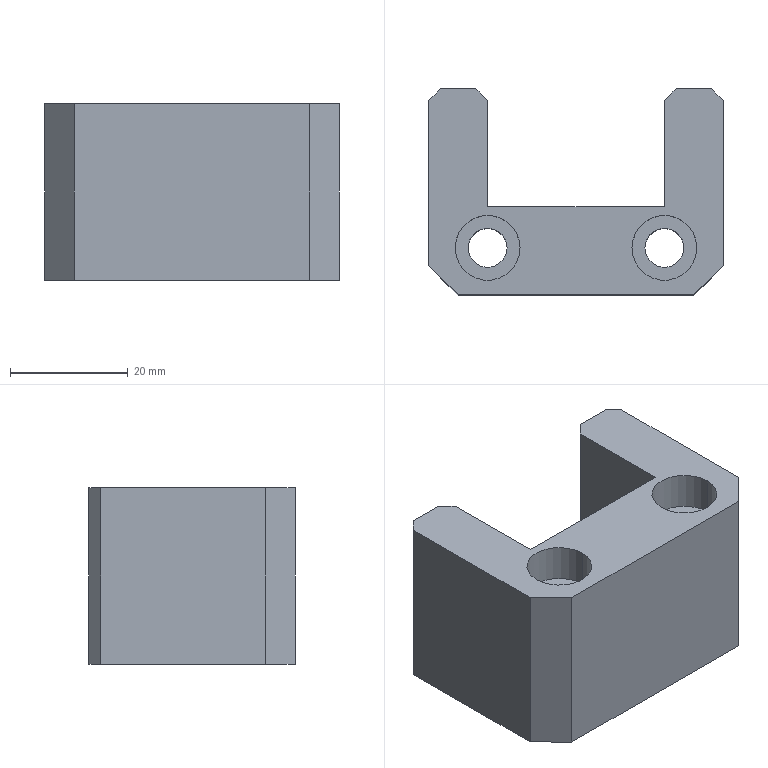Part | SolidWorks | features Chamfer 2, Extrusion 1, HoleWzd 1 | 1 solid | 26 faces | box 50 x 35 x 30 mm | volume 30679 mm3 | plane 18 | cylinder 8 | commonest cylinder face diameters 6.6 x4 11 x4
STEP:
#1=CARTESIAN_POINT('',(-20.5,-7.,23.6));
#2=VERTEX_POINT('',#1);
#3=CARTESIAN_POINT('',(-9.5,-7.,23.6));
#4=VERTEX_POINT('',#3);
#5=CARTESIAN_POINT('',(-15.,-7.,23.6));
#6=DIRECTION('',(0.,0.,1.));
#7=DIRECTION('',(1.,0.,0.));
#8=AXIS2_PLACEMENT_3D('',#5,#6,#7);
#9=CIRCLE('',#8,5.5);
#10=EDGE_CURVE('',#2,#4,#9,.T.);
#11=ORIENTED_EDGE('',*,*,#10,.F.);
#12=CARTESIAN_POINT('',(-20.5,-7.,30.));
#13=VERTEX_POINT('',#12);
#14=CARTESIAN_POINT('',(-20.5,-7.,30.));
#15=DIRECTION('',(0.,0.,1.));
#16=VECTOR('',#15,1000.);
#17=LINE('',#14,#16);
#18=EDGE_CURVE('',#2,#13,#17,.T.);
#19=ORIENTED_EDGE('',*,*,#18,.T.);
#20=CARTESIAN_POINT('',(-9.5,-7.,30.));
#21=VERTEX_POINT('',#20);
#22=CARTESIAN_POINT('',(-15.,-7.,30.));
#23=DIRECTION('',(0.,0.,1.));
#24=DIRECTION('',(1.,0.,0.));
#25=AXIS2_PLACEMENT_3D('',#22,#23,#24);
#26=CIRCLE('',#25,5.5);
#27=EDGE_CURVE('',#13,#21,#26,.T.);
#28=ORIENTED_EDGE('',*,*,#27,.T.);
#29=CARTESIAN_POINT('',(-9.5,-7.,30.));
#30=DIRECTION('',(0.,0.,1.));
#31=VECTOR('',#30,1000.);
#32=LINE('',#29,#31);
#33=EDGE_CURVE('',#4,#21,#32,.T.);
#34=ORIENTED_EDGE('',*,*,#33,.F.);
#35=EDGE_LOOP('',(#11,#19,#28,#34));
#36=FACE_OUTER_BOUND('',#35,.T.);
#37=CARTESIAN_POINT('',(-15.,-7.,30.));
#38=DIRECTION('',(0.,0.,1.));
#39=DIRECTION('',(1.,0.,0.));
#40=AXIS2_PLACEMENT_3D('',#37,#38,#39);
#41=CYLINDRICAL_SURFACE('',#40,5.5);
#42=ADVANCED_FACE('',(#36),#41,.F.);
#43=CARTESIAN_POINT('',(-18.3,-7.,0.));
#44=VERTEX_POINT('',#43);
#45=CARTESIAN_POINT('',(-11.7,-7.,0.));
#46=VERTEX_POINT('',#45);
#47=CARTESIAN_POINT('',(-15.,-7.,0.));
#48=DIRECTION('',(0.,0.,1.));
#49=DIRECTION('',(1.,0.,0.));
#50=AXIS2_PLACEMENT_3D('',#47,#48,#49);
#51=CIRCLE('',#50,3.3);
#52=EDGE_CURVE('',#44,#46,#51,.T.);
#53=ORIENTED_EDGE('',*,*,#52,.F.);
#54=CARTESIAN_POINT('',(-18.3,-7.,23.6));
#55=VERTEX_POINT('',#54);
#56=CARTESIAN_POINT('',(-18.3,-7.,30.));
#57=DIRECTION('',(0.,0.,1.));
#58=VECTOR('',#57,1000.);
#59=LINE('',#56,#58);
#60=EDGE_CURVE('',#44,#55,#59,.T.);
#61=ORIENTED_EDGE('',*,*,#60,.T.);
#62=CARTESIAN_POINT('',(-11.7,-7.,23.6));
#63=VERTEX_POINT('',#62);
#64=CARTESIAN_POINT('',(-15.,-7.,23.6));
#65=DIRECTION('',(0.,0.,1.));
#66=DIRECTION('',(1.,0.,0.));
#67=AXIS2_PLACEMENT_3D('',#64,#65,#66);
#68=CIRCLE('',#67,3.3);
#69=EDGE_CURVE('',#55,#63,#68,.T.);
#70=ORIENTED_EDGE('',*,*,#69,.T.);
#71=CARTESIAN_POINT('',(-11.7,-7.,30.));
#72=DIRECTION('',(0.,0.,1.));
#73=VECTOR('',#72,1000.);
#74=LINE('',#71,#73);
#75=EDGE_CURVE('',#46,#63,#74,.T.);
#76=ORIENTED_EDGE('',*,*,#75,.F.);
#77=EDGE_LOOP('',(#53,#61,#70,#76));
#78=FACE_OUTER_BOUND('',#77,.T.);
#79=CARTESIAN_POINT('',(-15.,-7.,30.));
#80=DIRECTION('',(0.,0.,1.));
#81=DIRECTION('',(1.,0.,0.));
#82=AXIS2_PLACEMENT_3D('',#79,#80,#81);
#83=CYLINDRICAL_SURFACE('',#82,3.3);
#84=ADVANCED_FACE('',(#78),#83,.F.);
#85=CARTESIAN_POINT('',(9.5,-7.,23.6));
#86=VERTEX_POINT('',#85);
#87=CARTESIAN_POINT('',(20.5,-7.,23.6));
#88=VERTEX_POINT('',#87);
#89=CARTESIAN_POINT('',(15.,-7.,23.6));
#90=DIRECTION('',(0.,0.,1.));
#91=DIRECTION('',(1.,0.,0.));
#92=AXIS2_PLACEMENT_3D('',#89,#90,#91);
#93=CIRCLE('',#92,5.5);
#94=EDGE_CURVE('',#86,#88,#93,.T.);
#95=ORIENTED_EDGE('',*,*,#94,.F.);
#96=CARTESIAN_POINT('',(9.5,-7.,30.));
#97=VERTEX_POINT('',#96);
#98=CARTESIAN_POINT('',(9.5,-7.,30.));
#99=DIRECTION('',(0.,0.,1.));
#100=VECTOR('',#99,1000.);
#101=LINE('',#98,#100);
#102=EDGE_CURVE('',#86,#97,#101,.T.);
#103=ORIENTED_EDGE('',*,*,#102,.T.);
#104=CARTESIAN_POINT('',(20.5,-7.,30.));
#105=VERTEX_POINT('',#104);
#106=CARTESIAN_POINT('',(15.,-7.,30.));
#107=DIRECTION('',(0.,0.,1.));
#108=DIRECTION('',(1.,0.,0.));
#109=AXIS2_PLACEMENT_3D('',#106,#107,#108);
#110=CIRCLE('',#109,5.5);
#111=EDGE_CURVE('',#97,#105,#110,.T.);
#112=ORIENTED_EDGE('',*,*,#111,.T.);
#113=CARTESIAN_POINT('',(20.5,-7.,30.));
#114=DIRECTION('',(0.,0.,1.));
#115=VECTOR('',#114,1000.);
#116=LINE('',#113,#115);
#117=EDGE_CURVE('',#88,#105,#116,.T.);
#118=ORIENTED_EDGE('',*,*,#117,.F.);
#119=EDGE_LOOP('',(#95,#103,#112,#118));
#120=FACE_OUTER_BOUND('',#119,.T.);
#121=CARTESIAN_POINT('',(15.,-7.,30.));
#122=DIRECTION('',(0.,0.,1.));
#123=DIRECTION('',(1.,0.,0.));
#124=AXIS2_PLACEMENT_3D('',#121,#122,#123);
#125=CYLINDRICAL_SURFACE('',#124,5.5);
#126=ADVANCED_FACE('',(#120),#125,.F.);
#127=CARTESIAN_POINT('',(11.7,-7.,0.));
#128=VERTEX_POINT('',#127);
#129=CARTESIAN_POINT('',(18.3,-7.,0.));
#130=VERTEX_POINT('',#129);
#131=CARTESIAN_POINT('',(15.,-7.,0.));
#132=DIRECTION('',(0.,0.,1.));
#133=DIRECTION('',(1.,0.,0.));
#134=AXIS2_PLACEMENT_3D('',#131,#132,#133);
#135=CIRCLE('',#134,3.3);
#136=EDGE_CURVE('',#128,#130,#135,.T.);
#137=ORIENTED_EDGE('',*,*,#136,.F.);
#138=CARTESIAN_POINT('',(11.7,-7.,23.6));
#139=VERTEX_POINT('',#138);
#140=CARTESIAN_POINT('',(11.7,-7.,30.));
#141=DIRECTION('',(0.,0.,1.));
#142=VECTOR('',#141,1000.);
#143=LINE('',#140,#142);
#144=EDGE_CURVE('',#128,#139,#143,.T.);
#145=ORIENTED_EDGE('',*,*,#144,.T.);
#146=CARTESIAN_POINT('',(18.3,-7.,23.6));
#147=VERTEX_POINT('',#146);
#148=CARTESIAN_POINT('',(15.,-7.,23.6));
#149=DIRECTION('',(0.,0.,1.));
#150=DIRECTION('',(1.,0.,0.));
#151=AXIS2_PLACEMENT_3D('',#148,#149,#150);
#152=CIRCLE('',#151,3.3);
#153=EDGE_CURVE('',#139,#147,#152,.T.);
#154=ORIENTED_EDGE('',*,*,#153,.T.);
#155=CARTESIAN_POINT('',(18.3,-7.,30.));
#156=DIRECTION('',(0.,0.,1.));
#157=VECTOR('',#156,1000.);
#158=LINE('',#155,#157);
#159=EDGE_CURVE('',#130,#147,#158,.T.);
#160=ORIENTED_EDGE('',*,*,#159,.F.);
#161=EDGE_LOOP('',(#137,#145,#154,#160));
#162=FACE_OUTER_BOUND('',#161,.T.);
#163=CARTESIAN_POINT('',(15.,-7.,30.));
#164=DIRECTION('',(0.,0.,1.));
#165=DIRECTION('',(1.,0.,0.));
#166=AXIS2_PLACEMENT_3D('',#163,#164,#165);
#167=CYLINDRICAL_SURFACE('',#166,3.3);
#168=ADVANCED_FACE('',(#162),#167,.F.);
#169=CARTESIAN_POINT('',(-25.,18.,0.));
#170=VERTEX_POINT('',#169);
#171=CARTESIAN_POINT('',(-25.,-10.,0.));
#172=VERTEX_POINT('',#171);
#173=CARTESIAN_POINT('',(-25.,-15.,0.));
#174=DIRECTION('',(0.,-1.,0.));
#175=VECTOR('',#174,1000.);
#176=LINE('',#173,#175);
#177=EDGE_CURVE('',#170,#172,#176,.T.);
#178=ORIENTED_EDGE('',*,*,#177,.T.);
#179=CARTESIAN_POINT('',(-25.,-10.,30.));
#180=VERTEX_POINT('',#179);
#181=CARTESIAN_POINT('',(-25.,-10.,30.));
#182=DIRECTION('',(0.,0.,1.));
#183=VECTOR('',#182,1000.);
#184=LINE('',#181,#183);
#185=EDGE_CURVE('',#172,#180,#184,.T.);
#186=ORIENTED_EDGE('',*,*,#185,.T.);
#187=CARTESIAN_POINT('',(-25.,18.,30.));
#188=VERTEX_POINT('',#187);
#189=CARTESIAN_POINT('',(-25.,-15.,30.));
#190=DIRECTION('',(0.,-1.,0.));
#191=VECTOR('',#190,1000.);
#192=LINE('',#189,#191);
#193=EDGE_CURVE('',#188,#180,#192,.T.);
#194=ORIENTED_EDGE('',*,*,#193,.F.);
#195=CARTESIAN_POINT('',(-25.,18.,30.));
#196=DIRECTION('',(0.,0.,-1.));
#197=VECTOR('',#196,1000.);
#198=LINE('',#195,#197);
#199=EDGE_CURVE('',#188,#170,#198,.T.);
#200=ORIENTED_EDGE('',*,*,#199,.T.);
#201=EDGE_LOOP('',(#178,#186,#194,#200));
#202=FACE_OUTER_BOUND('',#201,.T.);
#203=CARTESIAN_POINT('',(-25.,-15.,30.));
#204=DIRECTION('',(1.,0.,0.));
#205=DIRECTION('',(0.,1.,0.));
#206=AXIS2_PLACEMENT_3D('',#203,#204,#205);
#207=PLANE('',#206);
#208=ADVANCED_FACE('',(#202),#207,.F.);
#209=CARTESIAN_POINT('',(-20.,-15.,0.));
#210=VERTEX_POINT('',#209);
#211=CARTESIAN_POINT('',(20.,-15.,0.));
#212=VERTEX_POINT('',#211);
#213=CARTESIAN_POINT('',(25.,-15.,0.));
#214=DIRECTION('',(1.,0.,0.));
#215=VECTOR('',#214,1000.);
#216=LINE('',#213,#215);
#217=EDGE_CURVE('',#210,#212,#216,.T.);
#218=ORIENTED_EDGE('',*,*,#217,.T.);
#219=CARTESIAN_POINT('',(20.,-15.,30.));
#220=VERTEX_POINT('',#219);
#221=CARTESIAN_POINT('',(20.,-15.,30.));
#222=DIRECTION('',(0.,0.,1.));
#223=VECTOR('',#222,1000.);
#224=LINE('',#221,#223);
#225=EDGE_CURVE('',#212,#220,#224,.T.);
#226=ORIENTED_EDGE('',*,*,#225,.T.);
#227=CARTESIAN_POINT('',(-20.,-15.,30.));
#228=VERTEX_POINT('',#227);
#229=CARTESIAN_POINT('',(25.,-15.,30.));
#230=DIRECTION('',(1.,0.,0.));
#231=VECTOR('',#230,1000.);
#232=LINE('',#229,#231);
#233=EDGE_CURVE('',#228,#220,#232,.T.);
#234=ORIENTED_EDGE('',*,*,#233,.F.);
#235=CARTESIAN_POINT('',(-20.,-15.,30.));
#236=DIRECTION('',(0.,0.,-1.));
#237=VECTOR('',#236,1000.);
#238=LINE('',#235,#237);
#239=EDGE_CURVE('',#228,#210,#238,.T.);
#240=ORIENTED_EDGE('',*,*,#239,.T.);
#241=EDGE_LOOP('',(#218,#226,#234,#240));
#242=FACE_OUTER_BOUND('',#241,.T.);
#243=CARTESIAN_POINT('',(25.,-15.,30.));
#244=DIRECTION('',(0.,1.,0.));
#245=DIRECTION('',(0.,0.,1.));
#246=AXIS2_PLACEMENT_3D('',#243,#244,#245);
#247=PLANE('',#246);
#248=ADVANCED_FACE('',(#242),#247,.F.);
#249=CARTESIAN_POINT('',(25.,-10.,30.));
#250=VERTEX_POINT('',#249);
#251=CARTESIAN_POINT('',(25.,18.,30.));
#252=VERTEX_POINT('',#251);
#253=CARTESIAN_POINT('',(25.,20.,30.));
#254=DIRECTION('',(0.,1.,0.));
#255=VECTOR('',#254,1000.);
#256=LINE('',#253,#255);
#257=EDGE_CURVE('',#250,#252,#256,.T.);
#258=ORIENTED_EDGE('',*,*,#257,.F.);
#259=CARTESIAN_POINT('',(25.,-10.,0.));
#260=VERTEX_POINT('',#259);
#261=CARTESIAN_POINT('',(25.,-10.,30.));
#262=DIRECTION('',(0.,0.,-1.));
#263=VECTOR('',#262,1000.);
#264=LINE('',#261,#263);
#265=EDGE_CURVE('',#250,#260,#264,.T.);
#266=ORIENTED_EDGE('',*,*,#265,.T.);
#267=CARTESIAN_POINT('',(25.,18.,0.));
#268=VERTEX_POINT('',#267);
#269=CARTESIAN_POINT('',(25.,20.,0.));
#270=DIRECTION('',(0.,1.,0.));
#271=VECTOR('',#270,1000.);
#272=LINE('',#269,#271);
#273=EDGE_CURVE('',#260,#268,#272,.T.);
#274=ORIENTED_EDGE('',*,*,#273,.T.);
#275=CARTESIAN_POINT('',(25.,18.,30.));
#276=DIRECTION('',(0.,0.,1.));
#277=VECTOR('',#276,1000.);
#278=LINE('',#275,#277);
#279=EDGE_CURVE('',#268,#252,#278,.T.);
#280=ORIENTED_EDGE('',*,*,#279,.T.);
#281=EDGE_LOOP('',(#258,#266,#274,#280));
#282=FACE_OUTER_BOUND('',#281,.T.);
#283=CARTESIAN_POINT('',(25.,20.,30.));
#284=DIRECTION('',(-1.,0.,0.));
#285=DIRECTION('',(0.,-1.,0.));
#286=AXIS2_PLACEMENT_3D('',#283,#284,#285);
#287=PLANE('',#286);
#288=ADVANCED_FACE('',(#282),#287,.F.);
#289=CARTESIAN_POINT('',(23.,20.,30.));
#290=VERTEX_POINT('',#289);
#291=CARTESIAN_POINT('',(17.,20.,30.));
#292=VERTEX_POINT('',#291);
#293=CARTESIAN_POINT('',(15.,20.,30.));
#294=DIRECTION('',(-1.,0.,0.));
#295=VECTOR('',#294,1000.);
#296=LINE('',#293,#295);
#297=EDGE_CURVE('',#290,#292,#296,.T.);
#298=ORIENTED_EDGE('',*,*,#297,.F.);
#299=CARTESIAN_POINT('',(23.,20.,0.));
#300=VERTEX_POINT('',#299);
#301=CARTESIAN_POINT('',(23.,20.,30.));
#302=DIRECTION('',(0.,0.,-1.));
#303=VECTOR('',#302,1000.);
#304=LINE('',#301,#303);
#305=EDGE_CURVE('',#290,#300,#304,.T.);
#306=ORIENTED_EDGE('',*,*,#305,.T.);
#307=CARTESIAN_POINT('',(17.,20.,0.));
#308=VERTEX_POINT('',#307);
#309=CARTESIAN_POINT('',(15.,20.,0.));
#310=DIRECTION('',(-1.,0.,0.));
#311=VECTOR('',#310,1000.);
#312=LINE('',#309,#311);
#313=EDGE_CURVE('',#300,#308,#312,.T.);
#314=ORIENTED_EDGE('',*,*,#313,.T.);
#315=CARTESIAN_POINT('',(17.,20.,30.));
#316=DIRECTION('',(0.,0.,1.));
#317=VECTOR('',#316,1000.);
#318=LINE('',#315,#317);
#319=EDGE_CURVE('',#308,#292,#318,.T.);
#320=ORIENTED_EDGE('',*,*,#319,.T.);
#321=EDGE_LOOP('',(#298,#306,#314,#320));
#322=FACE_OUTER_BOUND('',#321,.T.);
#323=CARTESIAN_POINT('',(15.,20.,30.));
#324=DIRECTION('',(0.,-1.,0.));
#325=DIRECTION('',(0.,0.,-1.));
#326=AXIS2_PLACEMENT_3D('',#323,#324,#325);
#327=PLANE('',#326);
#328=ADVANCED_FACE('',(#322),#327,.F.);
#329=CARTESIAN_POINT('',(15.,18.,30.));
#330=VERTEX_POINT('',#329);
#331=CARTESIAN_POINT('',(15.,0.,30.));
#332=VERTEX_POINT('',#331);
#333=CARTESIAN_POINT('',(15.,0.,30.));
#334=DIRECTION('',(0.,-1.,0.));
#335=VECTOR('',#334,1000.);
#336=LINE('',#333,#335);
#337=EDGE_CURVE('',#330,#332,#336,.T.);
#338=ORIENTED_EDGE('',*,*,#337,.F.);
#339=CARTESIAN_POINT('',(15.,18.,0.));
#340=VERTEX_POINT('',#339);
#341=CARTESIAN_POINT('',(15.,18.,30.));
#342=DIRECTION('',(0.,0.,-1.));
#343=VECTOR('',#342,1000.);
#344=LINE('',#341,#343);
#345=EDGE_CURVE('',#330,#340,#344,.T.);
#346=ORIENTED_EDGE('',*,*,#345,.T.);
#347=CARTESIAN_POINT('',(15.,0.,0.));
#348=VERTEX_POINT('',#347);
#349=CARTESIAN_POINT('',(15.,0.,0.));
#350=DIRECTION('',(0.,-1.,0.));
#351=VECTOR('',#350,1000.);
#352=LINE('',#349,#351);
#353=EDGE_CURVE('',#340,#348,#352,.T.);
#354=ORIENTED_EDGE('',*,*,#353,.T.);
#355=CARTESIAN_POINT('',(15.,0.,30.));
#356=DIRECTION('',(0.,0.,-1.));
#357=VECTOR('',#356,1000.);
#358=LINE('',#355,#357);
#359=EDGE_CURVE('',#332,#348,#358,.T.);
#360=ORIENTED_EDGE('',*,*,#359,.F.);
#361=EDGE_LOOP('',(#338,#346,#354,#360));
#362=FACE_OUTER_BOUND('',#361,.T.);
#363=CARTESIAN_POINT('',(15.,0.,30.));
#364=DIRECTION('',(1.,0.,0.));
#365=DIRECTION('',(0.,1.,0.));
#366=AXIS2_PLACEMENT_3D('',#363,#364,#365);
#367=PLANE('',#366);
#368=ADVANCED_FACE('',(#362),#367,.F.);
#369=CARTESIAN_POINT('',(-15.,0.,0.));
#370=VERTEX_POINT('',#369);
#371=CARTESIAN_POINT('',(-15.,0.,0.));
#372=DIRECTION('',(-1.,0.,0.));
#373=VECTOR('',#372,1000.);
#374=LINE('',#371,#373);
#375=EDGE_CURVE('',#348,#370,#374,.T.);
#376=ORIENTED_EDGE('',*,*,#375,.T.);
#377=CARTESIAN_POINT('',(-15.,0.,30.));
#378=VERTEX_POINT('',#377);
#379=CARTESIAN_POINT('',(-15.,0.,30.));
#380=DIRECTION('',(0.,0.,-1.));
#381=VECTOR('',#380,1000.);
#382=LINE('',#379,#381);
#383=EDGE_CURVE('',#378,#370,#382,.T.);
#384=ORIENTED_EDGE('',*,*,#383,.F.);
#385=CARTESIAN_POINT('',(-15.,0.,30.));
#386=DIRECTION('',(-1.,0.,0.));
#387=VECTOR('',#386,1000.);
#388=LINE('',#385,#387);
#389=EDGE_CURVE('',#332,#378,#388,.T.);
#390=ORIENTED_EDGE('',*,*,#389,.F.);
#391=ORIENTED_EDGE('',*,*,#359,.T.);
#392=EDGE_LOOP('',(#376,#384,#390,#391));
#393=FACE_OUTER_BOUND('',#392,.T.);
#394=CARTESIAN_POINT('',(-15.,0.,30.));
#395=DIRECTION('',(0.,-1.,0.));
#396=DIRECTION('',(0.,0.,-1.));
#397=AXIS2_PLACEMENT_3D('',#394,#395,#396);
#398=PLANE('',#397);
#399=ADVANCED_FACE('',(#393),#398,.F.);
#400=CARTESIAN_POINT('',(-15.,18.,0.));
#401=VERTEX_POINT('',#400);
#402=CARTESIAN_POINT('',(-15.,20.,0.));
#403=DIRECTION('',(0.,1.,0.));
#404=VECTOR('',#403,1000.);
#405=LINE('',#402,#404);
#406=EDGE_CURVE('',#370,#401,#405,.T.);
#407=ORIENTED_EDGE('',*,*,#406,.T.);
#408=CARTESIAN_POINT('',(-15.,18.,30.));
#409=VERTEX_POINT('',#408);
#410=CARTESIAN_POINT('',(-15.,18.,30.));
#411=DIRECTION('',(0.,0.,1.));
#412=VECTOR('',#411,1000.);
#413=LINE('',#410,#412);
#414=EDGE_CURVE('',#401,#409,#413,.T.);
#415=ORIENTED_EDGE('',*,*,#414,.T.);
#416=CARTESIAN_POINT('',(-15.,20.,30.));
#417=DIRECTION('',(0.,1.,0.));
#418=VECTOR('',#417,1000.);
#419=LINE('',#416,#418);
#420=EDGE_CURVE('',#378,#409,#419,.T.);
#421=ORIENTED_EDGE('',*,*,#420,.F.);
#422=ORIENTED_EDGE('',*,*,#383,.T.);
#423=EDGE_LOOP('',(#407,#415,#421,#422));
#424=FACE_OUTER_BOUND('',#423,.T.);
#425=CARTESIAN_POINT('',(-15.,20.,30.));
#426=DIRECTION('',(-1.,0.,0.));
#427=DIRECTION('',(0.,-1.,0.));
#428=AXIS2_PLACEMENT_3D('',#425,#426,#427);
#429=PLANE('',#428);
#430=ADVANCED_FACE('',(#424),#429,.F.);
#431=CARTESIAN_POINT('',(-17.,20.,30.));
#432=VERTEX_POINT('',#431);
#433=CARTESIAN_POINT('',(-23.,20.,30.));
#434=VERTEX_POINT('',#433);
#435=CARTESIAN_POINT('',(-25.,20.,30.));
#436=DIRECTION('',(-1.,0.,0.));
#437=VECTOR('',#436,1000.);
#438=LINE('',#435,#437);
#439=EDGE_CURVE('',#432,#434,#438,.T.);
#440=ORIENTED_EDGE('',*,*,#439,.F.);
#441=CARTESIAN_POINT('',(-17.,20.,0.));
#442=VERTEX_POINT('',#441);
#443=CARTESIAN_POINT('',(-17.,20.,30.));
#444=DIRECTION('',(0.,0.,-1.));
#445=VECTOR('',#444,1000.);
#446=LINE('',#443,#445);
#447=EDGE_CURVE('',#432,#442,#446,.T.);
#448=ORIENTED_EDGE('',*,*,#447,.T.);
#449=CARTESIAN_POINT('',(-23.,20.,0.));
#450=VERTEX_POINT('',#449);
#451=CARTESIAN_POINT('',(-25.,20.,0.));
#452=DIRECTION('',(-1.,0.,0.));
#453=VECTOR('',#452,1000.);
#454=LINE('',#451,#453);
#455=EDGE_CURVE('',#442,#450,#454,.T.);
#456=ORIENTED_EDGE('',*,*,#455,.T.);
#457=CARTESIAN_POINT('',(-23.,20.,30.));
#458=DIRECTION('',(0.,0.,1.));
#459=VECTOR('',#458,1000.);
#460=LINE('',#457,#459);
#461=EDGE_CURVE('',#450,#434,#460,.T.);
#462=ORIENTED_EDGE('',*,*,#461,.T.);
#463=EDGE_LOOP('',(#440,#448,#456,#462));
#464=FACE_OUTER_BOUND('',#463,.T.);
#465=CARTESIAN_POINT('',(-25.,20.,30.));
#466=DIRECTION('',(0.,-1.,0.));
#467=DIRECTION('',(0.,0.,-1.));
#468=AXIS2_PLACEMENT_3D('',#465,#466,#467);
#469=PLANE('',#468);
#470=ADVANCED_FACE('',(#464),#469,.F.);
#471=CARTESIAN_POINT('',(-15.,-7.,30.));
#472=DIRECTION('',(0.,0.,1.));
#473=DIRECTION('',(1.,0.,0.));
#474=AXIS2_PLACEMENT_3D('',#471,#472,#473);
#475=CIRCLE('',#474,5.5);
#476=EDGE_CURVE('',#21,#13,#475,.T.);
#477=ORIENTED_EDGE('',*,*,#476,.F.);
#478=ORIENTED_EDGE('',*,*,#27,.F.);
#479=EDGE_LOOP('',(#477,#478));
#480=FACE_BOUND('',#479,.T.);
#481=CARTESIAN_POINT('',(15.,-7.,30.));
#482=DIRECTION('',(0.,0.,1.));
#483=DIRECTION('',(1.,0.,0.));
#484=AXIS2_PLACEMENT_3D('',#481,#482,#483);
#485=CIRCLE('',#484,5.5);
#486=EDGE_CURVE('',#105,#97,#485,.T.);
#487=ORIENTED_EDGE('',*,*,#486,.F.);
#488=ORIENTED_EDGE('',*,*,#111,.F.);
#489=EDGE_LOOP('',(#487,#488));
#490=FACE_BOUND('',#489,.T.);
#491=ORIENTED_EDGE('',*,*,#233,.T.);
#492=CARTESIAN_POINT('',(25.,-10.,30.));
#493=DIRECTION('',(0.7071,0.7071,0.));
#494=VECTOR('',#493,1000.);
#495=LINE('',#492,#494);
#496=EDGE_CURVE('',#220,#250,#495,.T.);
#497=ORIENTED_EDGE('',*,*,#496,.T.);
#498=ORIENTED_EDGE('',*,*,#257,.T.);
#499=CARTESIAN_POINT('',(23.,20.,30.));
#500=DIRECTION('',(-0.7071,0.7071,0.));
#501=VECTOR('',#500,1000.);
#502=LINE('',#499,#501);
#503=EDGE_CURVE('',#252,#290,#502,.T.);
#504=ORIENTED_EDGE('',*,*,#503,.T.);
#505=ORIENTED_EDGE('',*,*,#297,.T.);
#506=CARTESIAN_POINT('',(15.,18.,30.));
#507=DIRECTION('',(-0.7071,-0.7071,0.));
#508=VECTOR('',#507,1000.);
#509=LINE('',#506,#508);
#510=EDGE_CURVE('',#292,#330,#509,.T.);
#511=ORIENTED_EDGE('',*,*,#510,.T.);
#512=ORIENTED_EDGE('',*,*,#337,.T.);
#513=ORIENTED_EDGE('',*,*,#389,.T.);
#514=ORIENTED_EDGE('',*,*,#420,.T.);
#515=CARTESIAN_POINT('',(-17.,20.,30.));
#516=DIRECTION('',(-0.7071,0.7071,0.));
#517=VECTOR('',#516,1000.);
#518=LINE('',#515,#517);
#519=EDGE_CURVE('',#409,#432,#518,.T.);
#520=ORIENTED_EDGE('',*,*,#519,.T.);
#521=ORIENTED_EDGE('',*,*,#439,.T.);
#522=CARTESIAN_POINT('',(-25.,18.,30.));
#523=DIRECTION('',(-0.7071,-0.7071,0.));
#524=VECTOR('',#523,1000.);
#525=LINE('',#522,#524);
#526=EDGE_CURVE('',#434,#188,#525,.T.);
#527=ORIENTED_EDGE('',*,*,#526,.T.);
#528=ORIENTED_EDGE('',*,*,#193,.T.);
#529=CARTESIAN_POINT('',(-20.,-15.,30.));
#530=DIRECTION('',(0.7071,-0.7071,0.));
#531=VECTOR('',#530,1000.);
#532=LINE('',#529,#531);
#533=EDGE_CURVE('',#180,#228,#532,.T.);
#534=ORIENTED_EDGE('',*,*,#533,.T.);
#535=EDGE_LOOP('',(#491,#497,#498,#504,#505,#511,#512,#513,#514,#520,#521,#527,#528,#534));
#536=FACE_OUTER_BOUND('',#535,.T.);
#537=CARTESIAN_POINT('',(0.,0.,30.));
#538=DIRECTION('',(0.,0.,-1.));
#539=DIRECTION('',(-1.,0.,0.));
#540=AXIS2_PLACEMENT_3D('',#537,#538,#539);
#541=PLANE('',#540);
#542=ADVANCED_FACE('',(#480,#490,#536),#541,.F.);
#543=CARTESIAN_POINT('',(-15.,-7.,0.));
#544=DIRECTION('',(0.,0.,1.));
#545=DIRECTION('',(1.,0.,0.));
#546=AXIS2_PLACEMENT_3D('',#543,#544,#545);
#547=CIRCLE('',#546,3.3);
#548=EDGE_CURVE('',#46,#44,#547,.T.);
#549=ORIENTED_EDGE('',*,*,#548,.T.);
#550=ORIENTED_EDGE('',*,*,#52,.T.);
#551=EDGE_LOOP('',(#549,#550));
#552=FACE_BOUND('',#551,.T.);
#553=CARTESIAN_POINT('',(15.,-7.,0.));
#554=DIRECTION('',(0.,0.,1.));
#555=DIRECTION('',(1.,0.,0.));
#556=AXIS2_PLACEMENT_3D('',#553,#554,#555);
#557=CIRCLE('',#556,3.3);
#558=EDGE_CURVE('',#130,#128,#557,.T.);
#559=ORIENTED_EDGE('',*,*,#558,.T.);
#560=ORIENTED_EDGE('',*,*,#136,.T.);
#561=EDGE_LOOP('',(#559,#560));
#562=FACE_BOUND('',#561,.T.);
#563=ORIENTED_EDGE('',*,*,#273,.F.);
#564=CARTESIAN_POINT('',(17.5,-17.5,0.));
#565=DIRECTION('',(-0.7071,-0.7071,0.));
#566=VECTOR('',#565,1000.);
#567=LINE('',#564,#566);
#568=EDGE_CURVE('',#260,#212,#567,.T.);
#569=ORIENTED_EDGE('',*,*,#568,.T.);
#570=ORIENTED_EDGE('',*,*,#217,.F.);
#571=CARTESIAN_POINT('',(-17.5,-17.5,0.));
#572=DIRECTION('',(-0.7071,0.7071,0.));
#573=VECTOR('',#572,1000.);
#574=LINE('',#571,#573);
#575=EDGE_CURVE('',#210,#172,#574,.T.);
#576=ORIENTED_EDGE('',*,*,#575,.T.);
#577=ORIENTED_EDGE('',*,*,#177,.F.);
#578=CARTESIAN_POINT('',(-21.5,21.5,0.));
#579=DIRECTION('',(0.7071,0.7071,0.));
#580=VECTOR('',#579,1000.);
#581=LINE('',#578,#580);
#582=EDGE_CURVE('',#170,#450,#581,.T.);
#583=ORIENTED_EDGE('',*,*,#582,.T.);
#584=ORIENTED_EDGE('',*,*,#455,.F.);
#585=CARTESIAN_POINT('',(1.5,1.5,0.));
#586=DIRECTION('',(0.7071,-0.7071,0.));
#587=VECTOR('',#586,1000.);
#588=LINE('',#585,#587);
#589=EDGE_CURVE('',#442,#401,#588,.T.);
#590=ORIENTED_EDGE('',*,*,#589,.T.);
#591=ORIENTED_EDGE('',*,*,#406,.F.);
#592=ORIENTED_EDGE('',*,*,#375,.F.);
#593=ORIENTED_EDGE('',*,*,#353,.F.);
#594=CARTESIAN_POINT('',(-1.5,1.5,0.));
#595=DIRECTION('',(0.7071,0.7071,0.));
#596=VECTOR('',#595,1000.);
#597=LINE('',#594,#596);
#598=EDGE_CURVE('',#340,#308,#597,.T.);
#599=ORIENTED_EDGE('',*,*,#598,.T.);
#600=ORIENTED_EDGE('',*,*,#313,.F.);
#601=CARTESIAN_POINT('',(21.5,21.5,0.));
#602=DIRECTION('',(0.7071,-0.7071,0.));
#603=VECTOR('',#602,1000.);
#604=LINE('',#601,#603);
#605=EDGE_CURVE('',#300,#268,#604,.T.);
#606=ORIENTED_EDGE('',*,*,#605,.T.);
#607=EDGE_LOOP('',(#563,#569,#570,#576,#577,#583,#584,#590,#591,#592,#593,#599,#600,#606));
#608=FACE_OUTER_BOUND('',#607,.T.);
#609=CARTESIAN_POINT('',(0.,0.,0.));
#610=DIRECTION('',(0.,0.,-1.));
#611=DIRECTION('',(-1.,0.,0.));
#612=AXIS2_PLACEMENT_3D('',#609,#610,#611);
#613=PLANE('',#612);
#614=ADVANCED_FACE('',(#552,#562,#608),#613,.T.);
#615=ORIENTED_EDGE('',*,*,#144,.F.);
#616=ORIENTED_EDGE('',*,*,#558,.F.);
#617=ORIENTED_EDGE('',*,*,#159,.T.);
#618=CARTESIAN_POINT('',(15.,-7.,23.6));
#619=DIRECTION('',(0.,0.,1.));
#620=DIRECTION('',(1.,0.,0.));
#621=AXIS2_PLACEMENT_3D('',#618,#619,#620);
#622=CIRCLE('',#621,3.3);
#623=EDGE_CURVE('',#147,#139,#622,.T.);
#624=ORIENTED_EDGE('',*,*,#623,.T.);
#625=EDGE_LOOP('',(#615,#616,#617,#624));
#626=FACE_OUTER_BOUND('',#625,.T.);
#627=CARTESIAN_POINT('',(15.,-7.,30.));
#628=DIRECTION('',(0.,0.,1.));
#629=DIRECTION('',(1.,0.,0.));
#630=AXIS2_PLACEMENT_3D('',#627,#628,#629);
#631=CYLINDRICAL_SURFACE('',#630,3.3);
#632=ADVANCED_FACE('',(#626),#631,.F.);
#633=ORIENTED_EDGE('',*,*,#623,.F.);
#634=ORIENTED_EDGE('',*,*,#153,.F.);
#635=EDGE_LOOP('',(#633,#634));
#636=FACE_BOUND('',#635,.T.);
#637=CARTESIAN_POINT('',(15.,-7.,23.6));
#638=DIRECTION('',(0.,0.,1.));
#639=DIRECTION('',(1.,0.,0.));
#640=AXIS2_PLACEMENT_3D('',#637,#638,#639);
#641=CIRCLE('',#640,5.5);
#642=EDGE_CURVE('',#88,#86,#641,.T.);
#643=ORIENTED_EDGE('',*,*,#642,.T.);
#644=ORIENTED_EDGE('',*,*,#94,.T.);
#645=EDGE_LOOP('',(#643,#644));
#646=FACE_OUTER_BOUND('',#645,.T.);
#647=CARTESIAN_POINT('',(18.3,-7.,23.6));
#648=DIRECTION('',(0.,0.,-1.));
#649=DIRECTION('',(-1.,0.,0.));
#650=AXIS2_PLACEMENT_3D('',#647,#648,#649);
#651=PLANE('',#650);
#652=ADVANCED_FACE('',(#636,#646),#651,.F.);
#653=ORIENTED_EDGE('',*,*,#102,.F.);
#654=ORIENTED_EDGE('',*,*,#642,.F.);
#655=ORIENTED_EDGE('',*,*,#117,.T.);
#656=ORIENTED_EDGE('',*,*,#486,.T.);
#657=EDGE_LOOP('',(#653,#654,#655,#656));
#658=FACE_OUTER_BOUND('',#657,.T.);
#659=CARTESIAN_POINT('',(15.,-7.,30.));
#660=DIRECTION('',(0.,0.,1.));
#661=DIRECTION('',(1.,0.,0.));
#662=AXIS2_PLACEMENT_3D('',#659,#660,#661);
#663=CYLINDRICAL_SURFACE('',#662,5.5);
#664=ADVANCED_FACE('',(#658),#663,.F.);
#665=ORIENTED_EDGE('',*,*,#60,.F.);
#666=ORIENTED_EDGE('',*,*,#548,.F.);
#667=ORIENTED_EDGE('',*,*,#75,.T.);
#668=CARTESIAN_POINT('',(-15.,-7.,23.6));
#669=DIRECTION('',(0.,0.,1.));
#670=DIRECTION('',(1.,0.,0.));
#671=AXIS2_PLACEMENT_3D('',#668,#669,#670);
#672=CIRCLE('',#671,3.3);
#673=EDGE_CURVE('',#63,#55,#672,.T.);
#674=ORIENTED_EDGE('',*,*,#673,.T.);
#675=EDGE_LOOP('',(#665,#666,#667,#674));
#676=FACE_OUTER_BOUND('',#675,.T.);
#677=CARTESIAN_POINT('',(-15.,-7.,30.));
#678=DIRECTION('',(0.,0.,1.));
#679=DIRECTION('',(1.,0.,0.));
#680=AXIS2_PLACEMENT_3D('',#677,#678,#679);
#681=CYLINDRICAL_SURFACE('',#680,3.3);
#682=ADVANCED_FACE('',(#676),#681,.F.);
#683=ORIENTED_EDGE('',*,*,#673,.F.);
#684=ORIENTED_EDGE('',*,*,#69,.F.);
#685=EDGE_LOOP('',(#683,#684));
#686=FACE_BOUND('',#685,.T.);
#687=CARTESIAN_POINT('',(-15.,-7.,23.6));
#688=DIRECTION('',(0.,0.,1.));
#689=DIRECTION('',(1.,0.,0.));
#690=AXIS2_PLACEMENT_3D('',#687,#688,#689);
#691=CIRCLE('',#690,5.5);
#692=EDGE_CURVE('',#4,#2,#691,.T.);
#693=ORIENTED_EDGE('',*,*,#692,.T.);
#694=ORIENTED_EDGE('',*,*,#10,.T.);
#695=EDGE_LOOP('',(#693,#694));
#696=FACE_OUTER_BOUND('',#695,.T.);
#697=CARTESIAN_POINT('',(-11.7,-7.,23.6));
#698=DIRECTION('',(0.,0.,-1.));
#699=DIRECTION('',(-1.,0.,0.));
#700=AXIS2_PLACEMENT_3D('',#697,#698,#699);
#701=PLANE('',#700);
#702=ADVANCED_FACE('',(#686,#696),#701,.F.);
#703=ORIENTED_EDGE('',*,*,#18,.F.);
#704=ORIENTED_EDGE('',*,*,#692,.F.);
#705=ORIENTED_EDGE('',*,*,#33,.T.);
#706=ORIENTED_EDGE('',*,*,#476,.T.);
#707=EDGE_LOOP('',(#703,#704,#705,#706));
#708=FACE_OUTER_BOUND('',#707,.T.);
#709=CARTESIAN_POINT('',(-15.,-7.,30.));
#710=DIRECTION('',(0.,0.,1.));
#711=DIRECTION('',(1.,0.,0.));
#712=AXIS2_PLACEMENT_3D('',#709,#710,#711);
#713=CYLINDRICAL_SURFACE('',#712,5.5);
#714=ADVANCED_FACE('',(#708),#713,.F.);
#715=ORIENTED_EDGE('',*,*,#503,.F.);
#716=ORIENTED_EDGE('',*,*,#279,.F.);
#717=ORIENTED_EDGE('',*,*,#605,.F.);
#718=ORIENTED_EDGE('',*,*,#305,.F.);
#719=EDGE_LOOP('',(#715,#716,#717,#718));
#720=FACE_OUTER_BOUND('',#719,.T.);
#721=CARTESIAN_POINT('',(23.,20.,30.));
#722=DIRECTION('',(-0.7071,-0.7071,0.));
#723=DIRECTION('',(0.,0.,-1.));
#724=AXIS2_PLACEMENT_3D('',#721,#722,#723);
#725=PLANE('',#724);
#726=ADVANCED_FACE('',(#720),#725,.F.);
#727=ORIENTED_EDGE('',*,*,#510,.F.);
#728=ORIENTED_EDGE('',*,*,#319,.F.);
#729=ORIENTED_EDGE('',*,*,#598,.F.);
#730=ORIENTED_EDGE('',*,*,#345,.F.);
#731=EDGE_LOOP('',(#727,#728,#729,#730));
#732=FACE_OUTER_BOUND('',#731,.T.);
#733=CARTESIAN_POINT('',(15.,18.,30.));
#734=DIRECTION('',(0.7071,-0.7071,0.));
#735=DIRECTION('',(0.,0.,-1.));
#736=AXIS2_PLACEMENT_3D('',#733,#734,#735);
#737=PLANE('',#736);
#738=ADVANCED_FACE('',(#732),#737,.F.);
#739=ORIENTED_EDGE('',*,*,#519,.F.);
#740=ORIENTED_EDGE('',*,*,#414,.F.);
#741=ORIENTED_EDGE('',*,*,#589,.F.);
#742=ORIENTED_EDGE('',*,*,#447,.F.);
#743=EDGE_LOOP('',(#739,#740,#741,#742));
#744=FACE_OUTER_BOUND('',#743,.T.);
#745=CARTESIAN_POINT('',(-17.,20.,30.));
#746=DIRECTION('',(-0.7071,-0.7071,0.));
#747=DIRECTION('',(0.,0.,-1.));
#748=AXIS2_PLACEMENT_3D('',#745,#746,#747);
#749=PLANE('',#748);
#750=ADVANCED_FACE('',(#744),#749,.F.);
#751=ORIENTED_EDGE('',*,*,#526,.F.);
#752=ORIENTED_EDGE('',*,*,#461,.F.);
#753=ORIENTED_EDGE('',*,*,#582,.F.);
#754=ORIENTED_EDGE('',*,*,#199,.F.);
#755=EDGE_LOOP('',(#751,#752,#753,#754));
#756=FACE_OUTER_BOUND('',#755,.T.);
#757=CARTESIAN_POINT('',(-25.,18.,30.));
#758=DIRECTION('',(0.7071,-0.7071,0.));
#759=DIRECTION('',(0.,0.,-1.));
#760=AXIS2_PLACEMENT_3D('',#757,#758,#759);
#761=PLANE('',#760);
#762=ADVANCED_FACE('',(#756),#761,.F.);
#763=ORIENTED_EDGE('',*,*,#496,.F.);
#764=ORIENTED_EDGE('',*,*,#225,.F.);
#765=ORIENTED_EDGE('',*,*,#568,.F.);
#766=ORIENTED_EDGE('',*,*,#265,.F.);
#767=EDGE_LOOP('',(#763,#764,#765,#766));
#768=FACE_OUTER_BOUND('',#767,.T.);
#769=CARTESIAN_POINT('',(25.,-10.,30.));
#770=DIRECTION('',(-0.7071,0.7071,0.));
#771=DIRECTION('',(0.,0.,-1.));
#772=AXIS2_PLACEMENT_3D('',#769,#770,#771);
#773=PLANE('',#772);
#774=ADVANCED_FACE('',(#768),#773,.F.);
#775=ORIENTED_EDGE('',*,*,#533,.F.);
#776=ORIENTED_EDGE('',*,*,#185,.F.);
#777=ORIENTED_EDGE('',*,*,#575,.F.);
#778=ORIENTED_EDGE('',*,*,#239,.F.);
#779=EDGE_LOOP('',(#775,#776,#777,#778));
#780=FACE_OUTER_BOUND('',#779,.T.);
#781=CARTESIAN_POINT('',(-20.,-15.,30.));
#782=DIRECTION('',(0.7071,0.7071,0.));
#783=DIRECTION('',(0.,0.,-1.));
#784=AXIS2_PLACEMENT_3D('',#781,#782,#783);
#785=PLANE('',#784);
#786=ADVANCED_FACE('',(#780),#785,.F.);
#787=CLOSED_SHELL('',(#42,#84,#126,#168,#208,#248,#288,#328,#368,#399,#430,#470,#542,#614,#632,#652,#664,#682,#702,#714,#726,#738,#750,#762,#774,#786));
#788=MANIFOLD_SOLID_BREP('',#787);
#789=CARTESIAN_POINT('',(0.,0.,0.));
#790=DIRECTION('',(0.,0.,1.));
#791=DIRECTION('',(1.,0.,0.));
#792=AXIS2_PLACEMENT_3D('',#789,#790,#791);
#793=(LENGTH_UNIT()NAMED_UNIT(*)SI_UNIT(.MILLI.,.METRE.));
#794=UNCERTAINTY_MEASURE_WITH_UNIT(LENGTH_MEASURE(0.00001),#793,'','');
#795=(NAMED_UNIT(*)PLANE_ANGLE_UNIT()SI_UNIT($,.RADIAN.));
#796=(NAMED_UNIT(*)SI_UNIT($,.STERADIAN.)SOLID_ANGLE_UNIT());
#797=(GEOMETRIC_REPRESENTATION_CONTEXT(3)GLOBAL_UNCERTAINTY_ASSIGNED_CONTEXT((#794))GLOBAL_UNIT_ASSIGNED_CONTEXT((#793,#795,#796))REPRESENTATION_CONTEXT('',''));
#798=ADVANCED_BREP_SHAPE_REPRESENTATION('',(#788,#792),#797);